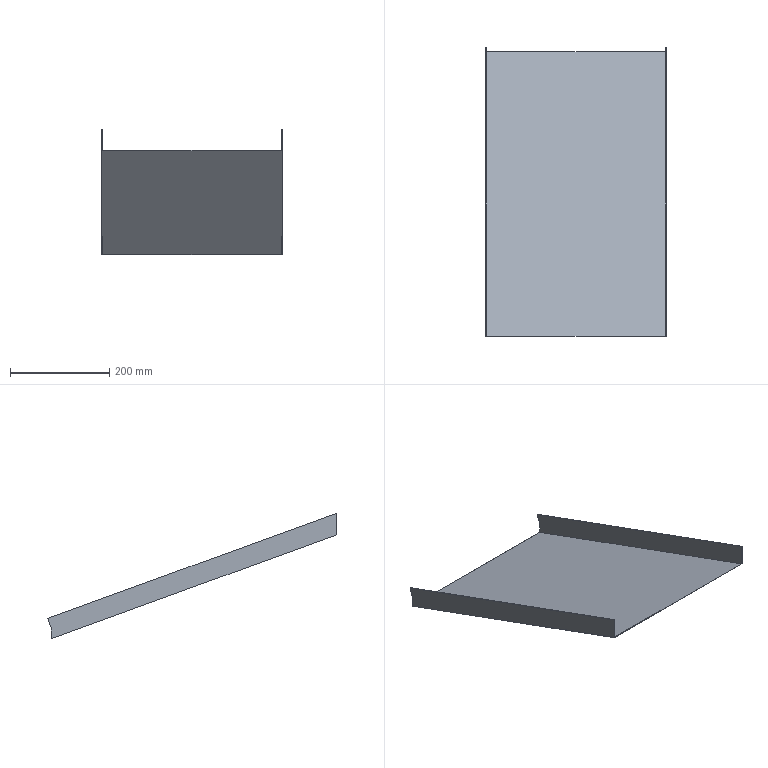Part | NX | features solid 2 | 1 solid | 12 faces | box 365 x 582.65 x 252.914 mm | volume 321613 mm3 | plane 12
STEP:
#1=CARTESIAN_POINT('',(-370.486,475.,-312.656));
#2=VERTEX_POINT('',#1);
#3=CARTESIAN_POINT('',(-731.486,475.,-312.656));
#4=VERTEX_POINT('',#3);
#5=CARTESIAN_POINT('',(-368.486,475.,-312.656));
#6=DIRECTION('',(-1.,0.,0.));
#7=VECTOR('',#6,1000.);
#8=LINE('',#5,#7);
#9=EDGE_CURVE('',#2,#4,#8,.T.);
#10=ORIENTED_EDGE('',*,*,#9,.F.);
#11=CARTESIAN_POINT('',(-370.486,1050.,-521.939));
#12=VERTEX_POINT('',#11);
#13=CARTESIAN_POINT('',(-370.486,121.685,-184.06));
#14=DIRECTION('',(0.,0.9397,-0.342));
#15=VECTOR('',#14,1000.);
#16=LINE('',#13,#15);
#17=EDGE_CURVE('',#2,#12,#16,.T.);
#18=ORIENTED_EDGE('',*,*,#17,.T.);
#19=CARTESIAN_POINT('',(-731.486,1050.,-521.939));
#20=VERTEX_POINT('',#19);
#21=CARTESIAN_POINT('',(-368.486,1050.,-521.939));
#22=DIRECTION('',(1.,0.,0.));
#23=VECTOR('',#22,1000.);
#24=LINE('',#21,#23);
#25=EDGE_CURVE('',#12,#20,#24,.F.);
#26=ORIENTED_EDGE('',*,*,#25,.T.);
#27=CARTESIAN_POINT('',(-731.486,121.685,-184.06));
#28=DIRECTION('',(0.,0.9397,-0.342));
#29=VECTOR('',#28,1000.);
#30=LINE('',#27,#29);
#31=EDGE_CURVE('',#4,#20,#30,.T.);
#32=ORIENTED_EDGE('',*,*,#31,.F.);
#33=EDGE_LOOP('',(#10,#18,#26,#32));
#34=FACE_BOUND('',#33,.T.);
#35=CARTESIAN_POINT('',(-368.486,496.391,-320.442));
#36=DIRECTION('',(0.,0.342,0.9397));
#37=DIRECTION('',(0.,-0.9397,0.342));
#38=AXIS2_PLACEMENT_3D('',#35,#36,#37);
#39=PLANE('',#38);
#40=ADVANCED_FACE('',(#34),#39,.T.);
#41=CARTESIAN_POINT('',(-733.486,475.,-270.089));
#42=VERTEX_POINT('',#41);
#43=CARTESIAN_POINT('',(-733.486,475.,-313.721));
#44=VERTEX_POINT('',#43);
#45=CARTESIAN_POINT('',(-733.486,475.,-321.382));
#46=DIRECTION('',(0.,0.,-1.));
#47=VECTOR('',#46,1000.);
#48=LINE('',#45,#47);
#49=EDGE_CURVE('',#42,#44,#48,.T.);
#50=ORIENTED_EDGE('',*,*,#49,.F.);
#51=CARTESIAN_POINT('',(-733.486,1057.65,-482.157));
#52=VERTEX_POINT('',#51);
#53=CARTESIAN_POINT('',(-733.486,135.366,-146.473));
#54=DIRECTION('',(0.,0.9397,-0.342));
#55=VECTOR('',#54,1000.);
#56=LINE('',#53,#55);
#57=EDGE_CURVE('',#42,#52,#56,.T.);
#58=ORIENTED_EDGE('',*,*,#57,.T.);
#59=CARTESIAN_POINT('',(-733.486,1050.,-503.175));
#60=VERTEX_POINT('',#59);
#61=CARTESIAN_POINT('',(-733.486,1057.65,-482.157));
#62=DIRECTION('',(0.,-0.342,-0.9397));
#63=VECTOR('',#62,1000.);
#64=LINE('',#61,#63);
#65=EDGE_CURVE('',#52,#60,#64,.T.);
#66=ORIENTED_EDGE('',*,*,#65,.T.);
#67=CARTESIAN_POINT('',(-733.486,1050.,-523.003));
#68=VERTEX_POINT('',#67);
#69=CARTESIAN_POINT('',(-733.486,1050.,-450.));
#70=DIRECTION('',(0.,0.,-1.));
#71=VECTOR('',#70,1000.);
#72=LINE('',#69,#71);
#73=EDGE_CURVE('',#68,#60,#72,.F.);
#74=ORIENTED_EDGE('',*,*,#73,.F.);
#75=CARTESIAN_POINT('',(-733.486,496.049,-321.382));
#76=DIRECTION('',(0.,0.9397,-0.342));
#77=VECTOR('',#76,1000.);
#78=LINE('',#75,#77);
#79=EDGE_CURVE('',#44,#68,#78,.T.);
#80=ORIENTED_EDGE('',*,*,#79,.F.);
#81=EDGE_LOOP('',(#50,#58,#66,#74,#80));
#82=FACE_BOUND('',#81,.T.);
#83=CARTESIAN_POINT('',(-733.486,496.049,-321.382));
#84=DIRECTION('',(-1.,0.,0.));
#85=DIRECTION('',(0.,1.,0.));
#86=AXIS2_PLACEMENT_3D('',#83,#84,#85);
#87=PLANE('',#86);
#88=ADVANCED_FACE('',(#82),#87,.T.);
#89=CARTESIAN_POINT('',(-368.486,1050.,-503.175));
#90=VERTEX_POINT('',#89);
#91=CARTESIAN_POINT('',(-370.486,1050.,-503.175));
#92=VERTEX_POINT('',#91);
#93=CARTESIAN_POINT('',(-368.486,1050.,-503.175));
#94=DIRECTION('',(-1.,0.,0.));
#95=VECTOR('',#94,1000.);
#96=LINE('',#93,#95);
#97=EDGE_CURVE('',#90,#92,#96,.T.);
#98=ORIENTED_EDGE('',*,*,#97,.F.);
#99=CARTESIAN_POINT('',(-368.486,1050.,-523.003));
#100=VERTEX_POINT('',#99);
#101=CARTESIAN_POINT('',(-368.486,1050.,-450.));
#102=DIRECTION('',(0.,0.,-1.));
#103=VECTOR('',#102,1000.);
#104=LINE('',#101,#103);
#105=EDGE_CURVE('',#100,#90,#104,.F.);
#106=ORIENTED_EDGE('',*,*,#105,.F.);
#107=CARTESIAN_POINT('',(-368.486,1050.,-523.003));
#108=DIRECTION('',(1.,0.,0.));
#109=VECTOR('',#108,1000.);
#110=LINE('',#107,#109);
#111=EDGE_CURVE('',#100,#68,#110,.F.);
#112=ORIENTED_EDGE('',*,*,#111,.T.);
#113=ORIENTED_EDGE('',*,*,#73,.T.);
#114=CARTESIAN_POINT('',(-731.486,1050.,-503.175));
#115=VERTEX_POINT('',#114);
#116=CARTESIAN_POINT('',(-733.486,1050.,-503.175));
#117=DIRECTION('',(-1.,0.,0.));
#118=VECTOR('',#117,1000.);
#119=LINE('',#116,#118);
#120=EDGE_CURVE('',#60,#115,#119,.F.);
#121=ORIENTED_EDGE('',*,*,#120,.T.);
#122=CARTESIAN_POINT('',(-731.486,1050.,-450.));
#123=DIRECTION('',(0.,0.,1.));
#124=VECTOR('',#123,1000.);
#125=LINE('',#122,#124);
#126=EDGE_CURVE('',#115,#20,#125,.F.);
#127=ORIENTED_EDGE('',*,*,#126,.T.);
#128=ORIENTED_EDGE('',*,*,#25,.F.);
#129=CARTESIAN_POINT('',(-370.486,1050.,-450.));
#130=DIRECTION('',(0.,0.,1.));
#131=VECTOR('',#130,1000.);
#132=LINE('',#129,#131);
#133=EDGE_CURVE('',#92,#12,#132,.F.);
#134=ORIENTED_EDGE('',*,*,#133,.F.);
#135=EDGE_LOOP('',(#98,#106,#112,#113,#121,#127,#128,#134));
#136=FACE_BOUND('',#135,.T.);
#137=CARTESIAN_POINT('',(750.,1050.,-450.));
#138=DIRECTION('',(0.,1.,0.));
#139=DIRECTION('',(1.,0.,0.));
#140=AXIS2_PLACEMENT_3D('',#137,#138,#139);
#141=PLANE('',#140);
#142=ADVANCED_FACE('',(#136),#141,.T.);
#143=CARTESIAN_POINT('',(-368.486,475.,-270.089));
#144=VERTEX_POINT('',#143);
#145=CARTESIAN_POINT('',(-368.486,1057.65,-482.157));
#146=VERTEX_POINT('',#145);
#147=CARTESIAN_POINT('',(-368.486,135.366,-146.473));
#148=DIRECTION('',(0.,0.9397,-0.342));
#149=VECTOR('',#148,1000.);
#150=LINE('',#147,#149);
#151=EDGE_CURVE('',#144,#146,#150,.T.);
#152=ORIENTED_EDGE('',*,*,#151,.F.);
#153=CARTESIAN_POINT('',(-368.486,475.,-313.721));
#154=VERTEX_POINT('',#153);
#155=CARTESIAN_POINT('',(-368.486,475.,-321.382));
#156=DIRECTION('',(0.,0.,-1.));
#157=VECTOR('',#156,1000.);
#158=LINE('',#155,#157);
#159=EDGE_CURVE('',#144,#154,#158,.T.);
#160=ORIENTED_EDGE('',*,*,#159,.T.);
#161=CARTESIAN_POINT('',(-368.486,496.049,-321.382));
#162=DIRECTION('',(0.,0.9397,-0.342));
#163=VECTOR('',#162,1000.);
#164=LINE('',#161,#163);
#165=EDGE_CURVE('',#154,#100,#164,.T.);
#166=ORIENTED_EDGE('',*,*,#165,.T.);
#167=ORIENTED_EDGE('',*,*,#105,.T.);
#168=CARTESIAN_POINT('',(-368.486,1043.627,-520.684));
#169=DIRECTION('',(0.,0.342,0.9397));
#170=VECTOR('',#169,1000.);
#171=LINE('',#168,#170);
#172=EDGE_CURVE('',#146,#90,#171,.F.);
#173=ORIENTED_EDGE('',*,*,#172,.F.);
#174=EDGE_LOOP('',(#152,#160,#166,#167,#173));
#175=FACE_BOUND('',#174,.T.);
#176=CARTESIAN_POINT('',(-368.486,496.049,-321.382));
#177=DIRECTION('',(-1.,0.,0.));
#178=DIRECTION('',(0.,0.,1.));
#179=AXIS2_PLACEMENT_3D('',#176,#177,#178);
#180=PLANE('',#179);
#181=ADVANCED_FACE('',(#175),#180,.F.);
#182=ORIENTED_EDGE('',*,*,#165,.F.);
#183=CARTESIAN_POINT('',(-368.486,475.,-313.721));
#184=DIRECTION('',(-1.,0.,0.));
#185=VECTOR('',#184,1000.);
#186=LINE('',#183,#185);
#187=EDGE_CURVE('',#154,#44,#186,.T.);
#188=ORIENTED_EDGE('',*,*,#187,.T.);
#189=ORIENTED_EDGE('',*,*,#79,.T.);
#190=ORIENTED_EDGE('',*,*,#111,.F.);
#191=EDGE_LOOP('',(#182,#188,#189,#190));
#192=FACE_BOUND('',#191,.T.);
#193=CARTESIAN_POINT('',(-368.486,496.049,-321.382));
#194=DIRECTION('',(0.,0.342,0.9397));
#195=DIRECTION('',(0.,-0.9397,0.342));
#196=AXIS2_PLACEMENT_3D('',#193,#194,#195);
#197=PLANE('',#196);
#198=ADVANCED_FACE('',(#192),#197,.F.);
#199=CARTESIAN_POINT('',(-731.486,475.,-270.089));
#200=VERTEX_POINT('',#199);
#201=CARTESIAN_POINT('',(-733.486,475.,-270.089));
#202=DIRECTION('',(-1.,0.,0.));
#203=VECTOR('',#202,1000.);
#204=LINE('',#201,#203);
#205=EDGE_CURVE('',#200,#42,#204,.T.);
#206=ORIENTED_EDGE('',*,*,#205,.F.);
#207=CARTESIAN_POINT('',(-731.486,1057.65,-482.157));
#208=VERTEX_POINT('',#207);
#209=CARTESIAN_POINT('',(-731.486,135.366,-146.473));
#210=DIRECTION('',(0.,0.9397,-0.342));
#211=VECTOR('',#210,1000.);
#212=LINE('',#209,#211);
#213=EDGE_CURVE('',#200,#208,#212,.T.);
#214=ORIENTED_EDGE('',*,*,#213,.T.);
#215=CARTESIAN_POINT('',(-733.486,1057.65,-482.157));
#216=DIRECTION('',(1.,0.,0.));
#217=VECTOR('',#216,1000.);
#218=LINE('',#215,#217);
#219=EDGE_CURVE('',#52,#208,#218,.T.);
#220=ORIENTED_EDGE('',*,*,#219,.F.);
#221=ORIENTED_EDGE('',*,*,#57,.F.);
#222=EDGE_LOOP('',(#206,#214,#220,#221));
#223=FACE_BOUND('',#222,.T.);
#224=CARTESIAN_POINT('',(-733.486,135.366,-146.473));
#225=DIRECTION('',(0.,0.342,0.9397));
#226=DIRECTION('',(0.,0.9397,-0.342));
#227=AXIS2_PLACEMENT_3D('',#224,#225,#226);
#228=PLANE('',#227);
#229=ADVANCED_FACE('',(#223),#228,.T.);
#230=ORIENTED_EDGE('',*,*,#219,.T.);
#231=CARTESIAN_POINT('',(-731.486,1057.65,-482.157));
#232=DIRECTION('',(0.,-0.342,-0.9397));
#233=VECTOR('',#232,1000.);
#234=LINE('',#231,#233);
#235=EDGE_CURVE('',#208,#115,#234,.T.);
#236=ORIENTED_EDGE('',*,*,#235,.T.);
#237=ORIENTED_EDGE('',*,*,#120,.F.);
#238=ORIENTED_EDGE('',*,*,#65,.F.);
#239=EDGE_LOOP('',(#230,#236,#237,#238));
#240=FACE_BOUND('',#239,.T.);
#241=CARTESIAN_POINT('',(-733.486,1057.65,-482.157));
#242=DIRECTION('',(0.,0.9397,-0.342));
#243=DIRECTION('',(0.,-0.342,-0.9397));
#244=AXIS2_PLACEMENT_3D('',#241,#242,#243);
#245=PLANE('',#244);
#246=ADVANCED_FACE('',(#240),#245,.T.);
#247=CARTESIAN_POINT('',(-731.486,475.,-146.473));
#248=DIRECTION('',(0.,0.,1.));
#249=VECTOR('',#248,1000.);
#250=LINE('',#247,#249);
#251=EDGE_CURVE('',#4,#200,#250,.T.);
#252=ORIENTED_EDGE('',*,*,#251,.F.);
#253=ORIENTED_EDGE('',*,*,#31,.T.);
#254=ORIENTED_EDGE('',*,*,#126,.F.);
#255=ORIENTED_EDGE('',*,*,#235,.F.);
#256=ORIENTED_EDGE('',*,*,#213,.F.);
#257=EDGE_LOOP('',(#252,#253,#254,#255,#256));
#258=FACE_BOUND('',#257,.T.);
#259=CARTESIAN_POINT('',(-731.486,135.366,-146.473));
#260=DIRECTION('',(1.,0.,0.));
#261=DIRECTION('',(0.,-1.,0.));
#262=AXIS2_PLACEMENT_3D('',#259,#260,#261);
#263=PLANE('',#262);
#264=ADVANCED_FACE('',(#258),#263,.T.);
#265=CARTESIAN_POINT('',(-370.486,475.,-270.089));
#266=VERTEX_POINT('',#265);
#267=CARTESIAN_POINT('',(-370.486,1057.65,-482.157));
#268=VERTEX_POINT('',#267);
#269=CARTESIAN_POINT('',(-370.486,135.366,-146.473));
#270=DIRECTION('',(0.,0.9397,-0.342));
#271=VECTOR('',#270,1000.);
#272=LINE('',#269,#271);
#273=EDGE_CURVE('',#266,#268,#272,.T.);
#274=ORIENTED_EDGE('',*,*,#273,.F.);
#275=CARTESIAN_POINT('',(-368.486,475.,-270.089));
#276=DIRECTION('',(-1.,0.,0.));
#277=VECTOR('',#276,1000.);
#278=LINE('',#275,#277);
#279=EDGE_CURVE('',#266,#144,#278,.F.);
#280=ORIENTED_EDGE('',*,*,#279,.T.);
#281=ORIENTED_EDGE('',*,*,#151,.T.);
#282=CARTESIAN_POINT('',(-368.486,1057.65,-482.157));
#283=DIRECTION('',(-1.,0.,0.));
#284=VECTOR('',#283,1000.);
#285=LINE('',#282,#284);
#286=EDGE_CURVE('',#146,#268,#285,.T.);
#287=ORIENTED_EDGE('',*,*,#286,.T.);
#288=EDGE_LOOP('',(#274,#280,#281,#287));
#289=FACE_BOUND('',#288,.T.);
#290=CARTESIAN_POINT('',(-368.486,135.366,-146.473));
#291=DIRECTION('',(0.,0.342,0.9397));
#292=DIRECTION('',(0.,0.9397,-0.342));
#293=AXIS2_PLACEMENT_3D('',#290,#291,#292);
#294=PLANE('',#293);
#295=ADVANCED_FACE('',(#289),#294,.T.);
#296=ORIENTED_EDGE('',*,*,#286,.F.);
#297=ORIENTED_EDGE('',*,*,#172,.T.);
#298=ORIENTED_EDGE('',*,*,#97,.T.);
#299=CARTESIAN_POINT('',(-370.486,1057.65,-482.157));
#300=DIRECTION('',(0.,0.342,0.9397));
#301=VECTOR('',#300,1000.);
#302=LINE('',#299,#301);
#303=EDGE_CURVE('',#268,#92,#302,.F.);
#304=ORIENTED_EDGE('',*,*,#303,.F.);
#305=EDGE_LOOP('',(#296,#297,#298,#304));
#306=FACE_BOUND('',#305,.T.);
#307=CARTESIAN_POINT('',(-368.486,1057.65,-482.157));
#308=DIRECTION('',(0.,0.9397,-0.342));
#309=DIRECTION('',(0.,-0.342,-0.9397));
#310=AXIS2_PLACEMENT_3D('',#307,#308,#309);
#311=PLANE('',#310);
#312=ADVANCED_FACE('',(#306),#311,.T.);
#313=ORIENTED_EDGE('',*,*,#17,.F.);
#314=CARTESIAN_POINT('',(-370.486,475.,-146.473));
#315=DIRECTION('',(0.,0.,1.));
#316=VECTOR('',#315,1000.);
#317=LINE('',#314,#316);
#318=EDGE_CURVE('',#2,#266,#317,.T.);
#319=ORIENTED_EDGE('',*,*,#318,.T.);
#320=ORIENTED_EDGE('',*,*,#273,.T.);
#321=ORIENTED_EDGE('',*,*,#303,.T.);
#322=ORIENTED_EDGE('',*,*,#133,.T.);
#323=EDGE_LOOP('',(#313,#319,#320,#321,#322));
#324=FACE_BOUND('',#323,.T.);
#325=CARTESIAN_POINT('',(-370.486,135.366,-146.473));
#326=DIRECTION('',(1.,0.,0.));
#327=DIRECTION('',(0.,0.,-1.));
#328=AXIS2_PLACEMENT_3D('',#325,#326,#327);
#329=PLANE('',#328);
#330=ADVANCED_FACE('',(#324),#329,.F.);
#331=ORIENTED_EDGE('',*,*,#205,.T.);
#332=ORIENTED_EDGE('',*,*,#49,.T.);
#333=ORIENTED_EDGE('',*,*,#187,.F.);
#334=ORIENTED_EDGE('',*,*,#159,.F.);
#335=ORIENTED_EDGE('',*,*,#279,.F.);
#336=ORIENTED_EDGE('',*,*,#318,.F.);
#337=ORIENTED_EDGE('',*,*,#9,.T.);
#338=ORIENTED_EDGE('',*,*,#251,.T.);
#339=EDGE_LOOP('',(#331,#332,#333,#334,#335,#336,#337,#338));
#340=FACE_BOUND('',#339,.T.);
#341=CARTESIAN_POINT('',(-765.,475.,-50.));
#342=DIRECTION('',(0.,1.,0.));
#343=DIRECTION('',(0.,0.,1.));
#344=AXIS2_PLACEMENT_3D('',#341,#342,#343);
#345=PLANE('',#344);
#346=ADVANCED_FACE('',(#340),#345,.F.);
#347=CLOSED_SHELL('',(#40,#88,#142,#181,#198,#229,#246,#264,#295,#312,#330,#346));
#348=MANIFOLD_SOLID_BREP('',#347);
#349=(LENGTH_UNIT()NAMED_UNIT(*)SI_UNIT(.MILLI.,.METRE.));
#350=UNCERTAINTY_MEASURE_WITH_UNIT(LENGTH_MEASURE(0.00001),#349,'','');
#351=(NAMED_UNIT(*)PLANE_ANGLE_UNIT()SI_UNIT($,.RADIAN.));
#352=(NAMED_UNIT(*)SI_UNIT($,.STERADIAN.)SOLID_ANGLE_UNIT());
#353=(GEOMETRIC_REPRESENTATION_CONTEXT(3)GLOBAL_UNCERTAINTY_ASSIGNED_CONTEXT((#350))GLOBAL_UNIT_ASSIGNED_CONTEXT((#349,#351,#352))REPRESENTATION_CONTEXT('',''));
#354=ADVANCED_BREP_SHAPE_REPRESENTATION('',(#348),#353);